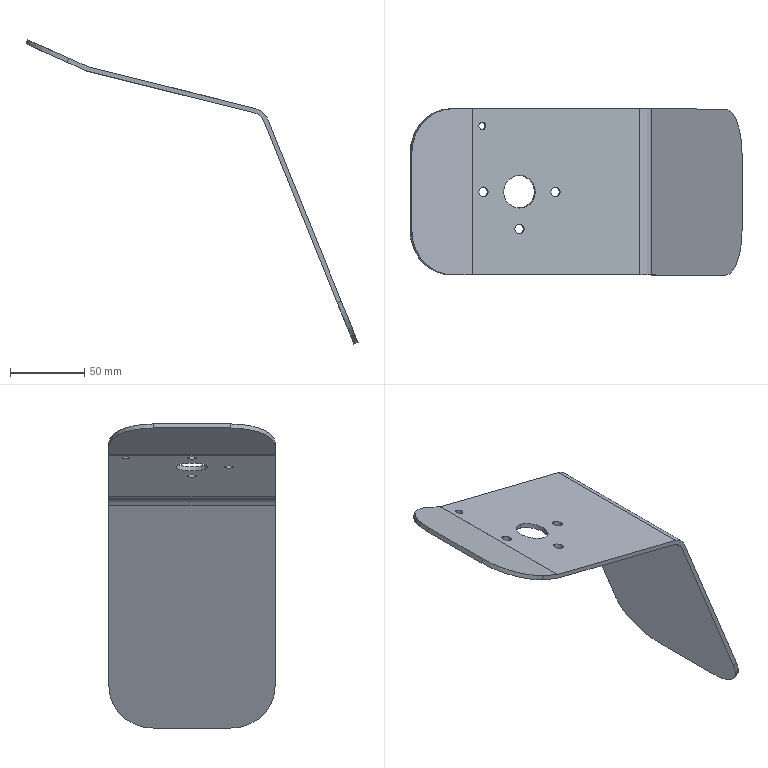Part | SolidWorks | features BaseBody 1 | 1 solid | 28 faces | box 223.764 x 112 x 205.006 mm | volume 108246 mm3 | cylinder 18 | plane 10 | commonest cylinder face diameters 6.5 x6 60 x4 5 x2 22 x2 2 x1 6 x1
STEP:
#1=CARTESIAN_POINT('',(-480.684,-15.,190.634));
#2=VERTEX_POINT('',#1);
#3=CARTESIAN_POINT('',(-480.684,7.,190.634));
#4=VERTEX_POINT('',#3);
#5=CARTESIAN_POINT('',(-480.684,-4.,190.634));
#6=DIRECTION('',(-0.2419,0.,-0.9703));
#7=DIRECTION('',(0.9703,0.,-0.2419));
#8=AXIS2_PLACEMENT_3D('',#5,#6,#7);
#9=CIRCLE('',#8,11.);
#10=EDGE_CURVE('',#2,#4,#9,.T.);
#11=ORIENTED_EDGE('',*,*,#10,.F.);
#12=CARTESIAN_POINT('',(-481.409,-15.,187.723));
#13=VERTEX_POINT('',#12);
#14=CARTESIAN_POINT('',(-481.409,-15.,187.723));
#15=DIRECTION('',(-0.2419,0.,-0.9703));
#16=VECTOR('',#15,1000.);
#17=LINE('',#14,#16);
#18=EDGE_CURVE('',#2,#13,#17,.T.);
#19=ORIENTED_EDGE('',*,*,#18,.T.);
#20=CARTESIAN_POINT('',(-481.409,7.,187.723));
#21=VERTEX_POINT('',#20);
#22=CARTESIAN_POINT('',(-481.409,-4.,187.723));
#23=DIRECTION('',(-0.2419,0.,-0.9703));
#24=DIRECTION('',(0.9703,0.,-0.2419));
#25=AXIS2_PLACEMENT_3D('',#22,#23,#24);
#26=CIRCLE('',#25,11.);
#27=EDGE_CURVE('',#13,#21,#26,.T.);
#28=ORIENTED_EDGE('',*,*,#27,.T.);
#29=CARTESIAN_POINT('',(-481.409,7.,187.723));
#30=DIRECTION('',(-0.2419,0.,-0.9703));
#31=VECTOR('',#30,1000.);
#32=LINE('',#29,#31);
#33=EDGE_CURVE('',#4,#21,#32,.T.);
#34=ORIENTED_EDGE('',*,*,#33,.F.);
#35=EDGE_LOOP('',(#11,#19,#28,#34));
#36=FACE_OUTER_BOUND('',#35,.T.);
#37=CARTESIAN_POINT('',(-481.409,-4.,187.723));
#38=DIRECTION('',(-0.2419,0.,-0.9703));
#39=DIRECTION('',(0.,1.,0.));
#40=AXIS2_PLACEMENT_3D('',#37,#38,#39);
#41=CYLINDRICAL_SURFACE('',#40,11.);
#42=ADVANCED_FACE('',(#36),#41,.F.);
#43=CARTESIAN_POINT('',(-456.426,-7.25,184.587));
#44=VERTEX_POINT('',#43);
#45=CARTESIAN_POINT('',(-456.426,-0.75,184.587));
#46=VERTEX_POINT('',#45);
#47=CARTESIAN_POINT('',(-456.426,-4.,184.587));
#48=DIRECTION('',(-0.2419,0.,-0.9703));
#49=DIRECTION('',(0.9703,0.,-0.2419));
#50=AXIS2_PLACEMENT_3D('',#47,#48,#49);
#51=CIRCLE('',#50,3.25);
#52=EDGE_CURVE('',#44,#46,#51,.T.);
#53=ORIENTED_EDGE('',*,*,#52,.F.);
#54=CARTESIAN_POINT('',(-457.152,-7.25,181.676));
#55=VERTEX_POINT('',#54);
#56=CARTESIAN_POINT('',(-457.152,-7.25,181.676));
#57=DIRECTION('',(-0.2419,0.,-0.9703));
#58=VECTOR('',#57,1000.);
#59=LINE('',#56,#58);
#60=EDGE_CURVE('',#44,#55,#59,.T.);
#61=ORIENTED_EDGE('',*,*,#60,.T.);
#62=CARTESIAN_POINT('',(-457.152,-0.75,181.676));
#63=VERTEX_POINT('',#62);
#64=CARTESIAN_POINT('',(-457.152,-4.,181.676));
#65=DIRECTION('',(-0.2419,0.,-0.9703));
#66=DIRECTION('',(0.9703,0.,-0.2419));
#67=AXIS2_PLACEMENT_3D('',#64,#65,#66);
#68=CIRCLE('',#67,3.25);
#69=EDGE_CURVE('',#55,#63,#68,.T.);
#70=ORIENTED_EDGE('',*,*,#69,.T.);
#71=CARTESIAN_POINT('',(-457.152,-0.75,181.676));
#72=DIRECTION('',(-0.2419,0.,-0.9703));
#73=VECTOR('',#72,1000.);
#74=LINE('',#71,#73);
#75=EDGE_CURVE('',#46,#63,#74,.T.);
#76=ORIENTED_EDGE('',*,*,#75,.F.);
#77=EDGE_LOOP('',(#53,#61,#70,#76));
#78=FACE_OUTER_BOUND('',#77,.T.);
#79=CARTESIAN_POINT('',(-457.152,-4.,181.676));
#80=DIRECTION('',(-0.2419,0.,-0.9703));
#81=DIRECTION('',(0.,1.,0.));
#82=AXIS2_PLACEMENT_3D('',#79,#80,#81);
#83=CYLINDRICAL_SURFACE('',#82,3.25);
#84=ADVANCED_FACE('',(#78),#83,.F.);
#85=CARTESIAN_POINT('',(-480.684,-32.25,190.634));
#86=VERTEX_POINT('',#85);
#87=CARTESIAN_POINT('',(-480.684,-25.75,190.634));
#88=VERTEX_POINT('',#87);
#89=CARTESIAN_POINT('',(-480.684,-29.,190.634));
#90=DIRECTION('',(-0.2419,0.,-0.9703));
#91=DIRECTION('',(0.9703,0.,-0.2419));
#92=AXIS2_PLACEMENT_3D('',#89,#90,#91);
#93=CIRCLE('',#92,3.25);
#94=EDGE_CURVE('',#86,#88,#93,.T.);
#95=ORIENTED_EDGE('',*,*,#94,.F.);
#96=CARTESIAN_POINT('',(-481.409,-32.25,187.723));
#97=VERTEX_POINT('',#96);
#98=CARTESIAN_POINT('',(-481.409,-32.25,187.723));
#99=DIRECTION('',(-0.2419,0.,-0.9703));
#100=VECTOR('',#99,1000.);
#101=LINE('',#98,#100);
#102=EDGE_CURVE('',#86,#97,#101,.T.);
#103=ORIENTED_EDGE('',*,*,#102,.T.);
#104=CARTESIAN_POINT('',(-481.409,-25.75,187.723));
#105=VERTEX_POINT('',#104);
#106=CARTESIAN_POINT('',(-481.409,-29.,187.723));
#107=DIRECTION('',(-0.2419,0.,-0.9703));
#108=DIRECTION('',(0.9703,0.,-0.2419));
#109=AXIS2_PLACEMENT_3D('',#106,#107,#108);
#110=CIRCLE('',#109,3.25);
#111=EDGE_CURVE('',#97,#105,#110,.T.);
#112=ORIENTED_EDGE('',*,*,#111,.T.);
#113=CARTESIAN_POINT('',(-481.409,-25.75,187.723));
#114=DIRECTION('',(-0.2419,0.,-0.9703));
#115=VECTOR('',#114,1000.);
#116=LINE('',#113,#115);
#117=EDGE_CURVE('',#88,#105,#116,.T.);
#118=ORIENTED_EDGE('',*,*,#117,.F.);
#119=EDGE_LOOP('',(#95,#103,#112,#118));
#120=FACE_OUTER_BOUND('',#119,.T.);
#121=CARTESIAN_POINT('',(-481.409,-29.,187.723));
#122=DIRECTION('',(-0.2419,0.,-0.9703));
#123=DIRECTION('',(0.,1.,0.));
#124=AXIS2_PLACEMENT_3D('',#121,#122,#123);
#125=CYLINDRICAL_SURFACE('',#124,3.25);
#126=ADVANCED_FACE('',(#120),#125,.F.);
#127=CARTESIAN_POINT('',(-504.941,-7.25,196.681));
#128=VERTEX_POINT('',#127);
#129=CARTESIAN_POINT('',(-504.941,-0.75,196.681));
#130=VERTEX_POINT('',#129);
#131=CARTESIAN_POINT('',(-504.941,-4.,196.681));
#132=DIRECTION('',(-0.2419,0.,-0.9703));
#133=DIRECTION('',(0.9703,0.,-0.2419));
#134=AXIS2_PLACEMENT_3D('',#131,#132,#133);
#135=CIRCLE('',#134,3.25);
#136=EDGE_CURVE('',#128,#130,#135,.T.);
#137=ORIENTED_EDGE('',*,*,#136,.F.);
#138=CARTESIAN_POINT('',(-505.667,-7.25,193.77));
#139=VERTEX_POINT('',#138);
#140=CARTESIAN_POINT('',(-505.667,-7.25,193.77));
#141=DIRECTION('',(-0.2419,0.,-0.9703));
#142=VECTOR('',#141,1000.);
#143=LINE('',#140,#142);
#144=EDGE_CURVE('',#128,#139,#143,.T.);
#145=ORIENTED_EDGE('',*,*,#144,.T.);
#146=CARTESIAN_POINT('',(-505.667,-0.75,193.77));
#147=VERTEX_POINT('',#146);
#148=CARTESIAN_POINT('',(-505.667,-4.,193.77));
#149=DIRECTION('',(-0.2419,0.,-0.9703));
#150=DIRECTION('',(0.9703,0.,-0.2419));
#151=AXIS2_PLACEMENT_3D('',#148,#149,#150);
#152=CIRCLE('',#151,3.25);
#153=EDGE_CURVE('',#139,#147,#152,.T.);
#154=ORIENTED_EDGE('',*,*,#153,.T.);
#155=CARTESIAN_POINT('',(-505.667,-0.75,193.77));
#156=DIRECTION('',(-0.2419,0.,-0.9703));
#157=VECTOR('',#156,1000.);
#158=LINE('',#155,#157);
#159=EDGE_CURVE('',#130,#147,#158,.T.);
#160=ORIENTED_EDGE('',*,*,#159,.F.);
#161=EDGE_LOOP('',(#137,#145,#154,#160));
#162=FACE_OUTER_BOUND('',#161,.T.);
#163=CARTESIAN_POINT('',(-505.667,-4.,193.77));
#164=DIRECTION('',(-0.2419,0.,-0.9703));
#165=DIRECTION('',(0.,1.,0.));
#166=AXIS2_PLACEMENT_3D('',#163,#164,#165);
#167=CYLINDRICAL_SURFACE('',#166,3.25);
#168=ADVANCED_FACE('',(#162),#167,.F.);
#169=CARTESIAN_POINT('',(-506.466,42.968,193.969));
#170=VERTEX_POINT('',#169);
#171=CARTESIAN_POINT('',(-506.466,37.968,193.969));
#172=VERTEX_POINT('',#171);
#173=CARTESIAN_POINT('',(-506.466,40.468,193.969));
#174=DIRECTION('',(0.2419,0.,0.9703));
#175=DIRECTION('',(0.,-1.,0.));
#176=AXIS2_PLACEMENT_3D('',#173,#174,#175);
#177=CIRCLE('',#176,2.5);
#178=EDGE_CURVE('',#170,#172,#177,.T.);
#179=ORIENTED_EDGE('',*,*,#178,.F.);
#180=CARTESIAN_POINT('',(-505.74,42.968,196.88));
#181=VERTEX_POINT('',#180);
#182=CARTESIAN_POINT('',(-508.159,42.968,187.177));
#183=DIRECTION('',(0.2419,0.,0.9703));
#184=VECTOR('',#183,1000.);
#185=LINE('',#182,#184);
#186=EDGE_CURVE('',#170,#181,#185,.T.);
#187=ORIENTED_EDGE('',*,*,#186,.T.);
#188=CARTESIAN_POINT('',(-505.74,37.968,196.88));
#189=VERTEX_POINT('',#188);
#190=CARTESIAN_POINT('',(-505.74,40.468,196.88));
#191=DIRECTION('',(-0.2419,0.,-0.9703));
#192=DIRECTION('',(0.,1.,0.));
#193=AXIS2_PLACEMENT_3D('',#190,#191,#192);
#194=CIRCLE('',#193,2.5);
#195=EDGE_CURVE('',#189,#181,#194,.T.);
#196=ORIENTED_EDGE('',*,*,#195,.F.);
#197=CARTESIAN_POINT('',(-508.159,37.968,187.177));
#198=DIRECTION('',(0.2419,0.,0.9703));
#199=VECTOR('',#198,1000.);
#200=LINE('',#197,#199);
#201=EDGE_CURVE('',#172,#189,#200,.T.);
#202=ORIENTED_EDGE('',*,*,#201,.F.);
#203=EDGE_LOOP('',(#179,#187,#196,#202));
#204=FACE_OUTER_BOUND('',#203,.T.);
#205=CARTESIAN_POINT('',(-508.159,40.468,187.177));
#206=DIRECTION('',(0.2419,0.,0.9703));
#207=DIRECTION('',(0.,-1.,0.));
#208=AXIS2_PLACEMENT_3D('',#205,#206,#207);
#209=CYLINDRICAL_SURFACE('',#208,2.5);
#210=ADVANCED_FACE('',(#204),#209,.F.);
#211=CARTESIAN_POINT('',(-399.786,52.,170.467));
#212=VERTEX_POINT('',#211);
#213=CARTESIAN_POINT('',(-391.563,52.,163.319));
#214=VERTEX_POINT('',#213);
#215=CARTESIAN_POINT('',(-402.689,52.,158.824));
#216=DIRECTION('',(0.,1.,0.));
#217=DIRECTION('',(0.,0.,1.));
#218=AXIS2_PLACEMENT_3D('',#215,#216,#217);
#219=CIRCLE('',#218,12.);
#220=EDGE_CURVE('',#212,#214,#219,.T.);
#221=ORIENTED_EDGE('',*,*,#220,.F.);
#222=CARTESIAN_POINT('',(-399.786,-60.,170.467));
#223=VERTEX_POINT('',#222);
#224=CARTESIAN_POINT('',(-399.786,46.,170.467));
#225=DIRECTION('',(0.,1.,0.));
#226=VECTOR('',#225,1000.);
#227=LINE('',#224,#226);
#228=EDGE_CURVE('',#223,#212,#227,.T.);
#229=ORIENTED_EDGE('',*,*,#228,.F.);
#230=CARTESIAN_POINT('',(-391.563,-60.,163.319));
#231=VERTEX_POINT('',#230);
#232=CARTESIAN_POINT('',(-402.689,-60.,158.824));
#233=DIRECTION('',(0.,-1.,0.));
#234=DIRECTION('',(0.,0.,-1.));
#235=AXIS2_PLACEMENT_3D('',#232,#233,#234);
#236=CIRCLE('',#235,12.);
#237=EDGE_CURVE('',#231,#223,#236,.T.);
#238=ORIENTED_EDGE('',*,*,#237,.F.);
#239=CARTESIAN_POINT('',(-391.563,-54.,163.319));
#240=DIRECTION('',(0.,-1.,0.));
#241=VECTOR('',#240,1000.);
#242=LINE('',#239,#241);
#243=EDGE_CURVE('',#214,#231,#242,.T.);
#244=ORIENTED_EDGE('',*,*,#243,.F.);
#245=EDGE_LOOP('',(#221,#229,#238,#244));
#246=FACE_OUTER_BOUND('',#245,.T.);
#247=CARTESIAN_POINT('',(-402.689,-4.,158.824));
#248=DIRECTION('',(0.,1.,0.));
#249=DIRECTION('',(0.,0.,-1.));
#250=AXIS2_PLACEMENT_3D('',#247,#248,#249);
#251=CYLINDRICAL_SURFACE('',#250,12.);
#252=ADVANCED_FACE('',(#246),#251,.T.);
#253=CARTESIAN_POINT('',(-394.153,52.,161.723));
#254=VERTEX_POINT('',#253);
#255=CARTESIAN_POINT('',(-401.006,52.,167.68));
#256=VERTEX_POINT('',#255);
#257=CARTESIAN_POINT('',(-403.425,52.,157.977));
#258=DIRECTION('',(0.,-1.,0.));
#259=DIRECTION('',(0.,0.,1.));
#260=AXIS2_PLACEMENT_3D('',#257,#258,#259);
#261=CIRCLE('',#260,10.);
#262=EDGE_CURVE('',#254,#256,#261,.T.);
#263=ORIENTED_EDGE('',*,*,#262,.F.);
#264=CARTESIAN_POINT('',(-394.153,-60.,161.723));
#265=VERTEX_POINT('',#264);
#266=CARTESIAN_POINT('',(-394.153,-4.,161.723));
#267=DIRECTION('',(0.,1.,0.));
#268=VECTOR('',#267,1000.);
#269=LINE('',#266,#268);
#270=EDGE_CURVE('',#265,#254,#269,.T.);
#271=ORIENTED_EDGE('',*,*,#270,.F.);
#272=CARTESIAN_POINT('',(-401.006,-60.,167.68));
#273=VERTEX_POINT('',#272);
#274=CARTESIAN_POINT('',(-403.425,-60.,157.977));
#275=DIRECTION('',(0.,1.,0.));
#276=DIRECTION('',(0.,0.,-1.));
#277=AXIS2_PLACEMENT_3D('',#274,#275,#276);
#278=CIRCLE('',#277,10.);
#279=EDGE_CURVE('',#273,#265,#278,.T.);
#280=ORIENTED_EDGE('',*,*,#279,.F.);
#281=CARTESIAN_POINT('',(-401.006,-4.,167.68));
#282=DIRECTION('',(0.,-1.,0.));
#283=VECTOR('',#282,1000.);
#284=LINE('',#281,#283);
#285=EDGE_CURVE('',#256,#273,#284,.T.);
#286=ORIENTED_EDGE('',*,*,#285,.F.);
#287=EDGE_LOOP('',(#263,#271,#280,#286));
#288=FACE_OUTER_BOUND('',#287,.T.);
#289=CARTESIAN_POINT('',(-403.425,-4.,157.977));
#290=DIRECTION('',(0.,-1.,0.));
#291=DIRECTION('',(0.,0.,1.));
#292=AXIS2_PLACEMENT_3D('',#289,#290,#291);
#293=CYLINDRICAL_SURFACE('',#292,10.);
#294=ADVANCED_FACE('',(#288),#293,.F.);
#295=CARTESIAN_POINT('',(-342.014,52.,40.681));
#296=VERTEX_POINT('',#295);
#297=CARTESIAN_POINT('',(-344.795,52.,39.557));
#298=VERTEX_POINT('',#297);
#299=CARTESIAN_POINT('',(-342.014,52.,40.681));
#300=DIRECTION('',(-0.9272,0.,-0.3746));
#301=VECTOR('',#300,1000.);
#302=LINE('',#299,#301);
#303=EDGE_CURVE('',#296,#298,#302,.T.);
#304=ORIENTED_EDGE('',*,*,#303,.F.);
#305=CARTESIAN_POINT('',(-330.776,22.,12.866));
#306=VERTEX_POINT('',#305);
#307=CARTESIAN_POINT('',(-342.014,22.,40.681));
#308=DIRECTION('',(0.9272,0.,0.3746));
#309=DIRECTION('',(0.3746,0.,-0.9272));
#310=AXIS2_PLACEMENT_3D('',#307,#308,#309);
#311=CIRCLE('',#310,30.);
#312=EDGE_CURVE('',#306,#296,#311,.T.);
#313=ORIENTED_EDGE('',*,*,#312,.F.);
#314=CARTESIAN_POINT('',(-333.557,22.,11.742));
#315=VERTEX_POINT('',#314);
#316=CARTESIAN_POINT('',(-330.776,22.,12.866));
#317=DIRECTION('',(-0.9272,0.,-0.3746));
#318=VECTOR('',#317,1000.);
#319=LINE('',#316,#318);
#320=EDGE_CURVE('',#306,#315,#319,.T.);
#321=ORIENTED_EDGE('',*,*,#320,.T.);
#322=CARTESIAN_POINT('',(-344.795,22.,39.557));
#323=DIRECTION('',(-0.9272,0.,-0.3746));
#324=DIRECTION('',(0.,1.,0.));
#325=AXIS2_PLACEMENT_3D('',#322,#323,#324);
#326=CIRCLE('',#325,30.);
#327=EDGE_CURVE('',#298,#315,#326,.T.);
#328=ORIENTED_EDGE('',*,*,#327,.F.);
#329=EDGE_LOOP('',(#304,#313,#321,#328));
#330=FACE_OUTER_BOUND('',#329,.T.);
#331=CARTESIAN_POINT('',(-341.087,22.,41.056));
#332=DIRECTION('',(-0.9272,0.,-0.3746));
#333=DIRECTION('',(0.3746,0.,-0.9272));
#334=AXIS2_PLACEMENT_3D('',#331,#332,#333);
#335=CYLINDRICAL_SURFACE('',#334,30.);
#336=ADVANCED_FACE('',(#330),#335,.T.);
#337=CARTESIAN_POINT('',(-333.557,-30.,11.742));
#338=VERTEX_POINT('',#337);
#339=CARTESIAN_POINT('',(-330.776,-30.,12.866));
#340=VERTEX_POINT('',#339);
#341=CARTESIAN_POINT('',(-333.557,-30.,11.742));
#342=DIRECTION('',(0.9272,0.,0.3746));
#343=VECTOR('',#342,1000.);
#344=LINE('',#341,#343);
#345=EDGE_CURVE('',#338,#340,#344,.T.);
#346=ORIENTED_EDGE('',*,*,#345,.F.);
#347=CARTESIAN_POINT('',(-333.557,-24.,11.742));
#348=DIRECTION('',(0.,1.,0.));
#349=VECTOR('',#348,1000.);
#350=LINE('',#347,#349);
#351=EDGE_CURVE('',#338,#315,#350,.T.);
#352=ORIENTED_EDGE('',*,*,#351,.T.);
#353=ORIENTED_EDGE('',*,*,#320,.F.);
#354=CARTESIAN_POINT('',(-330.776,-24.,12.866));
#355=DIRECTION('',(0.,1.,0.));
#356=VECTOR('',#355,1000.);
#357=LINE('',#354,#356);
#358=EDGE_CURVE('',#340,#306,#357,.T.);
#359=ORIENTED_EDGE('',*,*,#358,.F.);
#360=EDGE_LOOP('',(#346,#352,#353,#359));
#361=FACE_OUTER_BOUND('',#360,.T.);
#362=CARTESIAN_POINT('',(-329.848,36.,13.24));
#363=DIRECTION('',(-0.3746,0.,0.9272));
#364=DIRECTION('',(0.,1.,0.));
#365=AXIS2_PLACEMENT_3D('',#362,#363,#364);
#366=PLANE('',#365);
#367=ADVANCED_FACE('',(#361),#366,.F.);
#368=ORIENTED_EDGE('',*,*,#345,.T.);
#369=CARTESIAN_POINT('',(-342.014,-60.,40.681));
#370=VERTEX_POINT('',#369);
#371=CARTESIAN_POINT('',(-342.014,-30.,40.681));
#372=DIRECTION('',(0.9272,0.,0.3746));
#373=DIRECTION('',(0.,-1.,0.));
#374=AXIS2_PLACEMENT_3D('',#371,#372,#373);
#375=CIRCLE('',#374,30.);
#376=EDGE_CURVE('',#370,#340,#375,.T.);
#377=ORIENTED_EDGE('',*,*,#376,.F.);
#378=CARTESIAN_POINT('',(-344.795,-60.,39.557));
#379=VERTEX_POINT('',#378);
#380=CARTESIAN_POINT('',(-344.795,-60.,39.557));
#381=DIRECTION('',(0.9272,0.,0.3746));
#382=VECTOR('',#381,1000.);
#383=LINE('',#380,#382);
#384=EDGE_CURVE('',#379,#370,#383,.T.);
#385=ORIENTED_EDGE('',*,*,#384,.F.);
#386=CARTESIAN_POINT('',(-344.795,-30.,39.557));
#387=DIRECTION('',(-0.9272,0.,-0.3746));
#388=DIRECTION('',(0.3746,0.,-0.9272));
#389=AXIS2_PLACEMENT_3D('',#386,#387,#388);
#390=CIRCLE('',#389,30.);
#391=EDGE_CURVE('',#338,#379,#390,.T.);
#392=ORIENTED_EDGE('',*,*,#391,.F.);
#393=EDGE_LOOP('',(#368,#377,#385,#392));
#394=FACE_OUTER_BOUND('',#393,.T.);
#395=CARTESIAN_POINT('',(-345.478,-30.,39.281));
#396=DIRECTION('',(-0.9272,0.,-0.3746));
#397=DIRECTION('',(0.3746,0.,-0.9272));
#398=AXIS2_PLACEMENT_3D('',#395,#396,#397);
#399=CYLINDRICAL_SURFACE('',#398,30.);
#400=ADVANCED_FACE('',(#394),#399,.T.);
#401=CARTESIAN_POINT('',(-407.373,-60.,194.442));
#402=DIRECTION('',(0.3746,0.,-0.9272));
#403=VECTOR('',#402,1000.);
#404=LINE('',#401,#403);
#405=EDGE_CURVE('',#265,#379,#404,.T.);
#406=ORIENTED_EDGE('',*,*,#405,.F.);
#407=ORIENTED_EDGE('',*,*,#270,.T.);
#408=CARTESIAN_POINT('',(-407.373,52.,194.442));
#409=DIRECTION('',(-0.3746,0.,0.9272));
#410=VECTOR('',#409,1000.);
#411=LINE('',#408,#410);
#412=EDGE_CURVE('',#298,#254,#411,.T.);
#413=ORIENTED_EDGE('',*,*,#412,.F.);
#414=ORIENTED_EDGE('',*,*,#327,.T.);
#415=ORIENTED_EDGE('',*,*,#351,.F.);
#416=ORIENTED_EDGE('',*,*,#391,.T.);
#417=EDGE_LOOP('',(#406,#407,#413,#414,#415,#416));
#418=FACE_OUTER_BOUND('',#417,.T.);
#419=CARTESIAN_POINT('',(-367.152,-4.,94.893));
#420=DIRECTION('',(-0.9272,0.,-0.3746));
#421=DIRECTION('',(-0.3746,0.,0.9272));
#422=AXIS2_PLACEMENT_3D('',#419,#420,#421);
#423=PLANE('',#422);
#424=ADVANCED_FACE('',(#418),#423,.T.);
#425=CARTESIAN_POINT('',(-404.591,52.,195.566));
#426=DIRECTION('',(-0.3746,0.,0.9272));
#427=VECTOR('',#426,1000.);
#428=LINE('',#425,#427);
#429=EDGE_CURVE('',#296,#214,#428,.T.);
#430=ORIENTED_EDGE('',*,*,#429,.T.);
#431=ORIENTED_EDGE('',*,*,#243,.T.);
#432=CARTESIAN_POINT('',(-404.591,-60.,195.566));
#433=DIRECTION('',(0.3746,0.,-0.9272));
#434=VECTOR('',#433,1000.);
#435=LINE('',#432,#434);
#436=EDGE_CURVE('',#231,#370,#435,.T.);
#437=ORIENTED_EDGE('',*,*,#436,.T.);
#438=ORIENTED_EDGE('',*,*,#376,.T.);
#439=ORIENTED_EDGE('',*,*,#358,.T.);
#440=ORIENTED_EDGE('',*,*,#312,.T.);
#441=EDGE_LOOP('',(#430,#431,#437,#438,#439,#440));
#442=FACE_OUTER_BOUND('',#441,.T.);
#443=CARTESIAN_POINT('',(-401.535,-4.,188.003));
#444=DIRECTION('',(-0.9272,0.,-0.3746));
#445=DIRECTION('',(-0.3746,0.,0.9272));
#446=AXIS2_PLACEMENT_3D('',#443,#444,#445);
#447=PLANE('',#446);
#448=ADVANCED_FACE('',(#442),#447,.F.);
#449=CARTESIAN_POINT('',(-506.466,40.468,193.969));
#450=DIRECTION('',(0.2419,0.,0.9703));
#451=DIRECTION('',(0.,-1.,0.));
#452=AXIS2_PLACEMENT_3D('',#449,#450,#451);
#453=CIRCLE('',#452,2.5);
#454=EDGE_CURVE('',#172,#170,#453,.T.);
#455=ORIENTED_EDGE('',*,*,#454,.T.);
#456=ORIENTED_EDGE('',*,*,#178,.T.);
#457=EDGE_LOOP('',(#455,#456));
#458=FACE_BOUND('',#457,.T.);
#459=CARTESIAN_POINT('',(-505.667,-4.,193.77));
#460=DIRECTION('',(-0.2419,0.,-0.9703));
#461=DIRECTION('',(0.9703,0.,-0.2419));
#462=AXIS2_PLACEMENT_3D('',#459,#460,#461);
#463=CIRCLE('',#462,3.25);
#464=EDGE_CURVE('',#147,#139,#463,.T.);
#465=ORIENTED_EDGE('',*,*,#464,.F.);
#466=ORIENTED_EDGE('',*,*,#153,.F.);
#467=EDGE_LOOP('',(#465,#466));
#468=FACE_BOUND('',#467,.T.);
#469=CARTESIAN_POINT('',(-481.409,-29.,187.723));
#470=DIRECTION('',(-0.2419,0.,-0.9703));
#471=DIRECTION('',(0.9703,0.,-0.2419));
#472=AXIS2_PLACEMENT_3D('',#469,#470,#471);
#473=CIRCLE('',#472,3.25);
#474=EDGE_CURVE('',#105,#97,#473,.T.);
#475=ORIENTED_EDGE('',*,*,#474,.F.);
#476=ORIENTED_EDGE('',*,*,#111,.F.);
#477=EDGE_LOOP('',(#475,#476));
#478=FACE_BOUND('',#477,.T.);
#479=CARTESIAN_POINT('',(-457.152,-4.,181.676));
#480=DIRECTION('',(-0.2419,0.,-0.9703));
#481=DIRECTION('',(0.9703,0.,-0.2419));
#482=AXIS2_PLACEMENT_3D('',#479,#480,#481);
#483=CIRCLE('',#482,3.25);
#484=EDGE_CURVE('',#63,#55,#483,.T.);
#485=ORIENTED_EDGE('',*,*,#484,.F.);
#486=ORIENTED_EDGE('',*,*,#69,.F.);
#487=EDGE_LOOP('',(#485,#486));
#488=FACE_BOUND('',#487,.T.);
#489=CARTESIAN_POINT('',(-481.409,-4.,187.723));
#490=DIRECTION('',(-0.2419,0.,-0.9703));
#491=DIRECTION('',(0.9703,0.,-0.2419));
#492=AXIS2_PLACEMENT_3D('',#489,#490,#491);
#493=CIRCLE('',#492,11.);
#494=EDGE_CURVE('',#21,#13,#493,.T.);
#495=ORIENTED_EDGE('',*,*,#494,.F.);
#496=ORIENTED_EDGE('',*,*,#27,.F.);
#497=EDGE_LOOP('',(#495,#496));
#498=FACE_BOUND('',#497,.T.);
#499=CARTESIAN_POINT('',(-513.175,52.,195.642));
#500=VERTEX_POINT('',#499);
#501=CARTESIAN_POINT('',(-446.891,52.,179.118));
#502=DIRECTION('',(0.9703,0.,-0.2419));
#503=VECTOR('',#502,1000.);
#504=LINE('',#501,#503);
#505=EDGE_CURVE('',#500,#256,#504,.T.);
#506=ORIENTED_EDGE('',*,*,#505,.T.);
#507=ORIENTED_EDGE('',*,*,#285,.T.);
#508=CARTESIAN_POINT('',(-513.175,-60.,195.642));
#509=VERTEX_POINT('',#508);
#510=CARTESIAN_POINT('',(-446.891,-60.,179.118));
#511=DIRECTION('',(-0.9703,0.,0.2419));
#512=VECTOR('',#511,1000.);
#513=LINE('',#510,#512);
#514=EDGE_CURVE('',#273,#509,#513,.T.);
#515=ORIENTED_EDGE('',*,*,#514,.T.);
#516=CARTESIAN_POINT('',(-513.175,46.,195.642));
#517=DIRECTION('',(0.,-1.,0.));
#518=VECTOR('',#517,1000.);
#519=LINE('',#516,#518);
#520=EDGE_CURVE('',#500,#509,#519,.T.);
#521=ORIENTED_EDGE('',*,*,#520,.F.);
#522=EDGE_LOOP('',(#506,#507,#515,#521));
#523=FACE_OUTER_BOUND('',#522,.T.);
#524=CARTESIAN_POINT('',(-481.409,-4.,187.723));
#525=DIRECTION('',(0.2419,0.,0.9703));
#526=DIRECTION('',(0.,-1.,0.));
#527=AXIS2_PLACEMENT_3D('',#524,#525,#526);
#528=PLANE('',#527);
#529=ADVANCED_FACE('',(#458,#468,#478,#488,#498,#523),#528,.F.);
#530=ORIENTED_EDGE('',*,*,#195,.T.);
#531=CARTESIAN_POINT('',(-505.74,40.468,196.88));
#532=DIRECTION('',(-0.2419,0.,-0.9703));
#533=DIRECTION('',(0.,1.,0.));
#534=AXIS2_PLACEMENT_3D('',#531,#532,#533);
#535=CIRCLE('',#534,2.5);
#536=EDGE_CURVE('',#181,#189,#535,.T.);
#537=ORIENTED_EDGE('',*,*,#536,.T.);
#538=EDGE_LOOP('',(#530,#537));
#539=FACE_BOUND('',#538,.T.);
#540=CARTESIAN_POINT('',(-504.941,-4.,196.681));
#541=DIRECTION('',(-0.2419,0.,-0.9703));
#542=DIRECTION('',(0.9703,0.,-0.2419));
#543=AXIS2_PLACEMENT_3D('',#540,#541,#542);
#544=CIRCLE('',#543,3.25);
#545=EDGE_CURVE('',#130,#128,#544,.T.);
#546=ORIENTED_EDGE('',*,*,#545,.T.);
#547=ORIENTED_EDGE('',*,*,#136,.T.);
#548=EDGE_LOOP('',(#546,#547));
#549=FACE_BOUND('',#548,.T.);
#550=CARTESIAN_POINT('',(-480.684,-29.,190.634));
#551=DIRECTION('',(-0.2419,0.,-0.9703));
#552=DIRECTION('',(0.9703,0.,-0.2419));
#553=AXIS2_PLACEMENT_3D('',#550,#551,#552);
#554=CIRCLE('',#553,3.25);
#555=EDGE_CURVE('',#88,#86,#554,.T.);
#556=ORIENTED_EDGE('',*,*,#555,.T.);
#557=ORIENTED_EDGE('',*,*,#94,.T.);
#558=EDGE_LOOP('',(#556,#557));
#559=FACE_BOUND('',#558,.T.);
#560=CARTESIAN_POINT('',(-456.426,-4.,184.587));
#561=DIRECTION('',(-0.2419,0.,-0.9703));
#562=DIRECTION('',(0.9703,0.,-0.2419));
#563=AXIS2_PLACEMENT_3D('',#560,#561,#562);
#564=CIRCLE('',#563,3.25);
#565=EDGE_CURVE('',#46,#44,#564,.T.);
#566=ORIENTED_EDGE('',*,*,#565,.T.);
#567=ORIENTED_EDGE('',*,*,#52,.T.);
#568=EDGE_LOOP('',(#566,#567));
#569=FACE_BOUND('',#568,.T.);
#570=CARTESIAN_POINT('',(-480.684,-4.,190.634));
#571=DIRECTION('',(-0.2419,0.,-0.9703));
#572=DIRECTION('',(0.9703,0.,-0.2419));
#573=AXIS2_PLACEMENT_3D('',#570,#571,#572);
#574=CIRCLE('',#573,11.);
#575=EDGE_CURVE('',#4,#2,#574,.T.);
#576=ORIENTED_EDGE('',*,*,#575,.T.);
#577=ORIENTED_EDGE('',*,*,#10,.T.);
#578=EDGE_LOOP('',(#576,#577));
#579=FACE_BOUND('',#578,.T.);
#580=CARTESIAN_POINT('',(-512.364,-60.,198.531));
#581=VERTEX_POINT('',#580);
#582=CARTESIAN_POINT('',(-480.684,-60.,190.634));
#583=DIRECTION('',(0.9703,0.,-0.2419));
#584=VECTOR('',#583,1000.);
#585=LINE('',#582,#584);
#586=EDGE_CURVE('',#581,#223,#585,.T.);
#587=ORIENTED_EDGE('',*,*,#586,.T.);
#588=ORIENTED_EDGE('',*,*,#228,.T.);
#589=CARTESIAN_POINT('',(-512.364,52.,198.531));
#590=VERTEX_POINT('',#589);
#591=CARTESIAN_POINT('',(-480.684,52.,190.634));
#592=DIRECTION('',(-0.9703,0.,0.2419));
#593=VECTOR('',#592,1000.);
#594=LINE('',#591,#593);
#595=EDGE_CURVE('',#212,#590,#594,.T.);
#596=ORIENTED_EDGE('',*,*,#595,.T.);
#597=CARTESIAN_POINT('',(-512.364,-54.,198.531));
#598=DIRECTION('',(0.,1.,0.));
#599=VECTOR('',#598,1000.);
#600=LINE('',#597,#599);
#601=EDGE_CURVE('',#581,#590,#600,.T.);
#602=ORIENTED_EDGE('',*,*,#601,.F.);
#603=EDGE_LOOP('',(#587,#588,#596,#602));
#604=FACE_OUTER_BOUND('',#603,.T.);
#605=CARTESIAN_POINT('',(-480.684,-4.,190.634));
#606=DIRECTION('',(0.2419,0.,0.9703));
#607=DIRECTION('',(0.,-1.,0.));
#608=AXIS2_PLACEMENT_3D('',#605,#606,#607);
#609=PLANE('',#608);
#610=ADVANCED_FACE('',(#539,#549,#559,#569,#579,#604),#609,.T.);
#611=ORIENTED_EDGE('',*,*,#601,.T.);
#612=CARTESIAN_POINT('',(-512.529,52.,198.588));
#613=VERTEX_POINT('',#612);
#614=CARTESIAN_POINT('',(-512.122,52.,199.502));
#615=DIRECTION('',(0.,-1.,0.));
#616=DIRECTION('',(0.,0.,1.));
#617=AXIS2_PLACEMENT_3D('',#614,#615,#616);
#618=CIRCLE('',#617,1.);
#619=EDGE_CURVE('',#613,#590,#618,.T.);
#620=ORIENTED_EDGE('',*,*,#619,.F.);
#621=CARTESIAN_POINT('',(-512.529,-60.,198.588));
#622=VERTEX_POINT('',#621);
#623=CARTESIAN_POINT('',(-512.529,46.,198.588));
#624=DIRECTION('',(0.,-1.,0.));
#625=VECTOR('',#624,1000.);
#626=LINE('',#623,#625);
#627=EDGE_CURVE('',#613,#622,#626,.T.);
#628=ORIENTED_EDGE('',*,*,#627,.T.);
#629=CARTESIAN_POINT('',(-512.122,-60.,199.502));
#630=DIRECTION('',(0.,1.,0.));
#631=DIRECTION('',(0.,0.,-1.));
#632=AXIS2_PLACEMENT_3D('',#629,#630,#631);
#633=CIRCLE('',#632,1.);
#634=EDGE_CURVE('',#581,#622,#633,.T.);
#635=ORIENTED_EDGE('',*,*,#634,.F.);
#636=EDGE_LOOP('',(#611,#620,#628,#635));
#637=FACE_OUTER_BOUND('',#636,.T.);
#638=CARTESIAN_POINT('',(-512.122,-90.52,199.502));
#639=DIRECTION('',(0.,-1.,0.));
#640=DIRECTION('',(-0.9703,0.,0.2419));
#641=AXIS2_PLACEMENT_3D('',#638,#639,#640);
#642=CYLINDRICAL_SURFACE('',#641,1.);
#643=ADVANCED_FACE('',(#637),#642,.F.);
#644=CARTESIAN_POINT('',(-553.319,-30.,216.747));
#645=VERTEX_POINT('',#644);
#646=CARTESIAN_POINT('',(-525.913,-60.,204.546));
#647=VERTEX_POINT('',#646);
#648=CARTESIAN_POINT('',(-525.913,-30.,204.546));
#649=DIRECTION('',(0.4067,0.,0.9136));
#650=DIRECTION('',(-0.9136,0.,0.4067));
#651=AXIS2_PLACEMENT_3D('',#648,#649,#650);
#652=CIRCLE('',#651,30.);
#653=EDGE_CURVE('',#645,#647,#652,.T.);
#654=ORIENTED_EDGE('',*,*,#653,.T.);
#655=CARTESIAN_POINT('',(-450.397,-60.,170.928));
#656=DIRECTION('',(-0.9136,0.,0.4067));
#657=VECTOR('',#656,1000.);
#658=LINE('',#655,#657);
#659=EDGE_CURVE('',#622,#647,#658,.T.);
#660=ORIENTED_EDGE('',*,*,#659,.F.);
#661=ORIENTED_EDGE('',*,*,#627,.F.);
#662=CARTESIAN_POINT('',(-525.913,52.,204.546));
#663=VERTEX_POINT('',#662);
#664=CARTESIAN_POINT('',(-450.397,52.,170.928));
#665=DIRECTION('',(0.9136,0.,-0.4067));
#666=VECTOR('',#665,1000.);
#667=LINE('',#664,#666);
#668=EDGE_CURVE('',#663,#613,#667,.T.);
#669=ORIENTED_EDGE('',*,*,#668,.F.);
#670=CARTESIAN_POINT('',(-553.319,22.,216.747));
#671=VERTEX_POINT('',#670);
#672=CARTESIAN_POINT('',(-525.913,22.,204.546));
#673=DIRECTION('',(0.4067,0.,0.9136));
#674=DIRECTION('',(0.,1.,0.));
#675=AXIS2_PLACEMENT_3D('',#672,#673,#674);
#676=CIRCLE('',#675,30.);
#677=EDGE_CURVE('',#663,#671,#676,.T.);
#678=ORIENTED_EDGE('',*,*,#677,.T.);
#679=CARTESIAN_POINT('',(-553.319,16.,216.747));
#680=DIRECTION('',(0.,-1.,0.));
#681=VECTOR('',#680,1000.);
#682=LINE('',#679,#681);
#683=EDGE_CURVE('',#671,#645,#682,.T.);
#684=ORIENTED_EDGE('',*,*,#683,.T.);
#685=EDGE_LOOP('',(#654,#660,#661,#669,#678,#684));
#686=FACE_OUTER_BOUND('',#685,.T.);
#687=CARTESIAN_POINT('',(-512.209,-90.52,198.446));
#688=DIRECTION('',(0.4067,0.,0.9136));
#689=DIRECTION('',(0.,-1.,0.));
#690=AXIS2_PLACEMENT_3D('',#687,#688,#689);
#691=PLANE('',#690);
#692=ADVANCED_FACE('',(#686),#691,.T.);
#693=CARTESIAN_POINT('',(-554.54,-30.,214.007));
#694=VERTEX_POINT('',#693);
#695=CARTESIAN_POINT('',(-553.319,-30.,216.747));
#696=DIRECTION('',(-0.4067,0.,-0.9136));
#697=VECTOR('',#696,1000.);
#698=LINE('',#695,#697);
#699=EDGE_CURVE('',#645,#694,#698,.T.);
#700=ORIENTED_EDGE('',*,*,#699,.F.);
#701=ORIENTED_EDGE('',*,*,#683,.F.);
#702=CARTESIAN_POINT('',(-554.54,22.,214.007));
#703=VERTEX_POINT('',#702);
#704=CARTESIAN_POINT('',(-554.54,22.,214.007));
#705=DIRECTION('',(0.4067,0.,0.9136));
#706=VECTOR('',#705,1000.);
#707=LINE('',#704,#706);
#708=EDGE_CURVE('',#703,#671,#707,.T.);
#709=ORIENTED_EDGE('',*,*,#708,.F.);
#710=CARTESIAN_POINT('',(-554.54,16.,214.007));
#711=DIRECTION('',(0.,-1.,0.));
#712=VECTOR('',#711,1000.);
#713=LINE('',#710,#712);
#714=EDGE_CURVE('',#703,#694,#713,.T.);
#715=ORIENTED_EDGE('',*,*,#714,.T.);
#716=EDGE_LOOP('',(#700,#701,#709,#715));
#717=FACE_OUTER_BOUND('',#716,.T.);
#718=CARTESIAN_POINT('',(-552.913,-90.52,217.661));
#719=DIRECTION('',(-0.9136,0.,0.4067));
#720=DIRECTION('',(0.,1.,0.));
#721=AXIS2_PLACEMENT_3D('',#718,#719,#720);
#722=PLANE('',#721);
#723=ADVANCED_FACE('',(#717),#722,.T.);
#724=CARTESIAN_POINT('',(-527.133,-60.,201.806));
#725=VERTEX_POINT('',#724);
#726=CARTESIAN_POINT('',(-527.133,-30.,201.806));
#727=DIRECTION('',(-0.4067,0.,-0.9136));
#728=DIRECTION('',(0.,-1.,0.));
#729=AXIS2_PLACEMENT_3D('',#726,#727,#728);
#730=CIRCLE('',#729,30.);
#731=EDGE_CURVE('',#725,#694,#730,.T.);
#732=ORIENTED_EDGE('',*,*,#731,.T.);
#733=ORIENTED_EDGE('',*,*,#714,.F.);
#734=CARTESIAN_POINT('',(-527.133,52.,201.806));
#735=VERTEX_POINT('',#734);
#736=CARTESIAN_POINT('',(-527.133,22.,201.806));
#737=DIRECTION('',(-0.4067,0.,-0.9136));
#738=DIRECTION('',(-0.9136,0.,0.4067));
#739=AXIS2_PLACEMENT_3D('',#736,#737,#738);
#740=CIRCLE('',#739,30.);
#741=EDGE_CURVE('',#703,#735,#740,.T.);
#742=ORIENTED_EDGE('',*,*,#741,.T.);
#743=CARTESIAN_POINT('',(-513.669,52.,195.812));
#744=VERTEX_POINT('',#743);
#745=CARTESIAN_POINT('',(-451.617,52.,168.188));
#746=DIRECTION('',(-0.9136,0.,0.4067));
#747=VECTOR('',#746,1000.);
#748=LINE('',#745,#747);
#749=EDGE_CURVE('',#744,#735,#748,.T.);
#750=ORIENTED_EDGE('',*,*,#749,.F.);
#751=CARTESIAN_POINT('',(-513.669,-60.,195.812));
#752=VERTEX_POINT('',#751);
#753=CARTESIAN_POINT('',(-513.669,-54.,195.812));
#754=DIRECTION('',(0.,1.,0.));
#755=VECTOR('',#754,1000.);
#756=LINE('',#753,#755);
#757=EDGE_CURVE('',#752,#744,#756,.T.);
#758=ORIENTED_EDGE('',*,*,#757,.F.);
#759=CARTESIAN_POINT('',(-451.617,-60.,168.188));
#760=DIRECTION('',(0.9136,0.,-0.4067));
#761=VECTOR('',#760,1000.);
#762=LINE('',#759,#761);
#763=EDGE_CURVE('',#725,#752,#762,.T.);
#764=ORIENTED_EDGE('',*,*,#763,.F.);
#765=EDGE_LOOP('',(#732,#733,#742,#750,#758,#764));
#766=FACE_OUTER_BOUND('',#765,.T.);
#767=CARTESIAN_POINT('',(-513.429,-90.52,195.705));
#768=DIRECTION('',(-0.4067,0.,-0.9136));
#769=DIRECTION('',(-0.9136,0.,0.4067));
#770=AXIS2_PLACEMENT_3D('',#767,#768,#769);
#771=PLANE('',#770);
#772=ADVANCED_FACE('',(#766),#771,.T.);
#773=ORIENTED_EDGE('',*,*,#520,.T.);
#774=CARTESIAN_POINT('',(-512.449,-60.,198.553));
#775=DIRECTION('',(0.,-1.,0.));
#776=DIRECTION('',(0.,0.,-1.));
#777=AXIS2_PLACEMENT_3D('',#774,#775,#776);
#778=CIRCLE('',#777,3.);
#779=EDGE_CURVE('',#752,#509,#778,.T.);
#780=ORIENTED_EDGE('',*,*,#779,.F.);
#781=ORIENTED_EDGE('',*,*,#757,.T.);
#782=CARTESIAN_POINT('',(-512.449,52.,198.553));
#783=DIRECTION('',(0.,1.,0.));
#784=DIRECTION('',(0.,0.,1.));
#785=AXIS2_PLACEMENT_3D('',#782,#783,#784);
#786=CIRCLE('',#785,3.);
#787=EDGE_CURVE('',#500,#744,#786,.T.);
#788=ORIENTED_EDGE('',*,*,#787,.F.);
#789=EDGE_LOOP('',(#773,#780,#781,#788));
#790=FACE_OUTER_BOUND('',#789,.T.);
#791=CARTESIAN_POINT('',(-512.449,-90.52,198.553));
#792=DIRECTION('',(0.,1.,0.));
#793=DIRECTION('',(0.9703,0.,-0.2419));
#794=AXIS2_PLACEMENT_3D('',#791,#792,#793);
#795=CYLINDRICAL_SURFACE('',#794,3.);
#796=ADVANCED_FACE('',(#790),#795,.T.);
#797=ORIENTED_EDGE('',*,*,#708,.T.);
#798=ORIENTED_EDGE('',*,*,#677,.F.);
#799=CARTESIAN_POINT('',(-527.133,52.,201.806));
#800=DIRECTION('',(0.4067,0.,0.9136));
#801=VECTOR('',#800,1000.);
#802=LINE('',#799,#801);
#803=EDGE_CURVE('',#735,#663,#802,.T.);
#804=ORIENTED_EDGE('',*,*,#803,.F.);
#805=ORIENTED_EDGE('',*,*,#741,.F.);
#806=EDGE_LOOP('',(#797,#798,#804,#805));
#807=FACE_OUTER_BOUND('',#806,.T.);
#808=CARTESIAN_POINT('',(-522.585,22.,212.022));
#809=DIRECTION('',(0.4067,0.,0.9136));
#810=DIRECTION('',(-0.9136,0.,0.4067));
#811=AXIS2_PLACEMENT_3D('',#808,#809,#810);
#812=CYLINDRICAL_SURFACE('',#811,30.);
#813=ADVANCED_FACE('',(#807),#812,.T.);
#814=ORIENTED_EDGE('',*,*,#699,.T.);
#815=ORIENTED_EDGE('',*,*,#731,.F.);
#816=CARTESIAN_POINT('',(-525.913,-60.,204.546));
#817=DIRECTION('',(-0.4067,0.,-0.9136));
#818=VECTOR('',#817,1000.);
#819=LINE('',#816,#818);
#820=EDGE_CURVE('',#647,#725,#819,.T.);
#821=ORIENTED_EDGE('',*,*,#820,.F.);
#822=ORIENTED_EDGE('',*,*,#653,.F.);
#823=EDGE_LOOP('',(#814,#815,#821,#822));
#824=FACE_OUTER_BOUND('',#823,.T.);
#825=CARTESIAN_POINT('',(-522.585,-30.,212.022));
#826=DIRECTION('',(-0.4067,0.,-0.9136));
#827=DIRECTION('',(0.9136,0.,-0.4067));
#828=AXIS2_PLACEMENT_3D('',#825,#826,#827);
#829=CYLINDRICAL_SURFACE('',#828,30.);
#830=ADVANCED_FACE('',(#824),#829,.T.);
#831=ORIENTED_EDGE('',*,*,#186,.F.);
#832=ORIENTED_EDGE('',*,*,#454,.F.);
#833=ORIENTED_EDGE('',*,*,#201,.T.);
#834=ORIENTED_EDGE('',*,*,#536,.F.);
#835=EDGE_LOOP('',(#831,#832,#833,#834));
#836=FACE_OUTER_BOUND('',#835,.T.);
#837=CARTESIAN_POINT('',(-508.159,40.468,187.177));
#838=DIRECTION('',(0.2419,0.,0.9703));
#839=DIRECTION('',(0.,-1.,0.));
#840=AXIS2_PLACEMENT_3D('',#837,#838,#839);
#841=CYLINDRICAL_SURFACE('',#840,2.5);
#842=ADVANCED_FACE('',(#836),#841,.F.);
#843=ORIENTED_EDGE('',*,*,#144,.F.);
#844=ORIENTED_EDGE('',*,*,#545,.F.);
#845=ORIENTED_EDGE('',*,*,#159,.T.);
#846=ORIENTED_EDGE('',*,*,#464,.T.);
#847=EDGE_LOOP('',(#843,#844,#845,#846));
#848=FACE_OUTER_BOUND('',#847,.T.);
#849=CARTESIAN_POINT('',(-505.667,-4.,193.77));
#850=DIRECTION('',(-0.2419,0.,-0.9703));
#851=DIRECTION('',(0.,1.,0.));
#852=AXIS2_PLACEMENT_3D('',#849,#850,#851);
#853=CYLINDRICAL_SURFACE('',#852,3.25);
#854=ADVANCED_FACE('',(#848),#853,.F.);
#855=ORIENTED_EDGE('',*,*,#102,.F.);
#856=ORIENTED_EDGE('',*,*,#555,.F.);
#857=ORIENTED_EDGE('',*,*,#117,.T.);
#858=ORIENTED_EDGE('',*,*,#474,.T.);
#859=EDGE_LOOP('',(#855,#856,#857,#858));
#860=FACE_OUTER_BOUND('',#859,.T.);
#861=CARTESIAN_POINT('',(-481.409,-29.,187.723));
#862=DIRECTION('',(-0.2419,0.,-0.9703));
#863=DIRECTION('',(0.,1.,0.));
#864=AXIS2_PLACEMENT_3D('',#861,#862,#863);
#865=CYLINDRICAL_SURFACE('',#864,3.25);
#866=ADVANCED_FACE('',(#860),#865,.F.);
#867=ORIENTED_EDGE('',*,*,#60,.F.);
#868=ORIENTED_EDGE('',*,*,#565,.F.);
#869=ORIENTED_EDGE('',*,*,#75,.T.);
#870=ORIENTED_EDGE('',*,*,#484,.T.);
#871=EDGE_LOOP('',(#867,#868,#869,#870));
#872=FACE_OUTER_BOUND('',#871,.T.);
#873=CARTESIAN_POINT('',(-457.152,-4.,181.676));
#874=DIRECTION('',(-0.2419,0.,-0.9703));
#875=DIRECTION('',(0.,1.,0.));
#876=AXIS2_PLACEMENT_3D('',#873,#874,#875);
#877=CYLINDRICAL_SURFACE('',#876,3.25);
#878=ADVANCED_FACE('',(#872),#877,.F.);
#879=ORIENTED_EDGE('',*,*,#18,.F.);
#880=ORIENTED_EDGE('',*,*,#575,.F.);
#881=ORIENTED_EDGE('',*,*,#33,.T.);
#882=ORIENTED_EDGE('',*,*,#494,.T.);
#883=EDGE_LOOP('',(#879,#880,#881,#882));
#884=FACE_OUTER_BOUND('',#883,.T.);
#885=CARTESIAN_POINT('',(-481.409,-4.,187.723));
#886=DIRECTION('',(-0.2419,0.,-0.9703));
#887=DIRECTION('',(0.,1.,0.));
#888=AXIS2_PLACEMENT_3D('',#885,#886,#887);
#889=CYLINDRICAL_SURFACE('',#888,11.);
#890=ADVANCED_FACE('',(#884),#889,.F.);
#891=ORIENTED_EDGE('',*,*,#436,.F.);
#892=ORIENTED_EDGE('',*,*,#237,.T.);
#893=ORIENTED_EDGE('',*,*,#586,.F.);
#894=ORIENTED_EDGE('',*,*,#634,.T.);
#895=ORIENTED_EDGE('',*,*,#659,.T.);
#896=ORIENTED_EDGE('',*,*,#820,.T.);
#897=ORIENTED_EDGE('',*,*,#763,.T.);
#898=ORIENTED_EDGE('',*,*,#779,.T.);
#899=ORIENTED_EDGE('',*,*,#514,.F.);
#900=ORIENTED_EDGE('',*,*,#279,.T.);
#901=ORIENTED_EDGE('',*,*,#405,.T.);
#902=ORIENTED_EDGE('',*,*,#384,.T.);
#903=EDGE_LOOP('',(#891,#892,#893,#894,#895,#896,#897,#898,#899,#900,#901,#902));
#904=FACE_OUTER_BOUND('',#903,.T.);
#905=CARTESIAN_POINT('',(-447.069,-60.,178.403));
#906=DIRECTION('',(0.,-1.,0.));
#907=DIRECTION('',(0.,0.,-1.));
#908=AXIS2_PLACEMENT_3D('',#905,#906,#907);
#909=PLANE('',#908);
#910=ADVANCED_FACE('',(#904),#909,.T.);
#911=ORIENTED_EDGE('',*,*,#595,.F.);
#912=ORIENTED_EDGE('',*,*,#220,.T.);
#913=ORIENTED_EDGE('',*,*,#429,.F.);
#914=ORIENTED_EDGE('',*,*,#303,.T.);
#915=ORIENTED_EDGE('',*,*,#412,.T.);
#916=ORIENTED_EDGE('',*,*,#262,.T.);
#917=ORIENTED_EDGE('',*,*,#505,.F.);
#918=ORIENTED_EDGE('',*,*,#787,.T.);
#919=ORIENTED_EDGE('',*,*,#749,.T.);
#920=ORIENTED_EDGE('',*,*,#803,.T.);
#921=ORIENTED_EDGE('',*,*,#668,.T.);
#922=ORIENTED_EDGE('',*,*,#619,.T.);
#923=EDGE_LOOP('',(#911,#912,#913,#914,#915,#916,#917,#918,#919,#920,#921,#922));
#924=FACE_OUTER_BOUND('',#923,.T.);
#925=CARTESIAN_POINT('',(-447.069,52.,178.403));
#926=DIRECTION('',(0.,1.,0.));
#927=DIRECTION('',(1.,0.,0.));
#928=AXIS2_PLACEMENT_3D('',#925,#926,#927);
#929=PLANE('',#928);
#930=ADVANCED_FACE('',(#924),#929,.T.);
#931=CLOSED_SHELL('',(#42,#84,#126,#168,#210,#252,#294,#336,#367,#400,#424,#448,#529,#610,#643,#692,#723,#772,#796,#813,#830,#842,#854,#866,#878,#890,#910,#930));
#932=MANIFOLD_SOLID_BREP('',#931);
#933=CARTESIAN_POINT('',(0.,0.,0.));
#934=DIRECTION('',(0.,0.,1.));
#935=DIRECTION('',(1.,0.,0.));
#936=AXIS2_PLACEMENT_3D('',#933,#934,#935);
#937=(LENGTH_UNIT()NAMED_UNIT(*)SI_UNIT(.MILLI.,.METRE.));
#938=UNCERTAINTY_MEASURE_WITH_UNIT(LENGTH_MEASURE(0.00001),#937,'','');
#939=(NAMED_UNIT(*)PLANE_ANGLE_UNIT()SI_UNIT($,.RADIAN.));
#940=(NAMED_UNIT(*)SI_UNIT($,.STERADIAN.)SOLID_ANGLE_UNIT());
#941=(GEOMETRIC_REPRESENTATION_CONTEXT(3)GLOBAL_UNCERTAINTY_ASSIGNED_CONTEXT((#938))GLOBAL_UNIT_ASSIGNED_CONTEXT((#937,#939,#940))REPRESENTATION_CONTEXT('',''));
#942=ADVANCED_BREP_SHAPE_REPRESENTATION('',(#932,#936),#941);